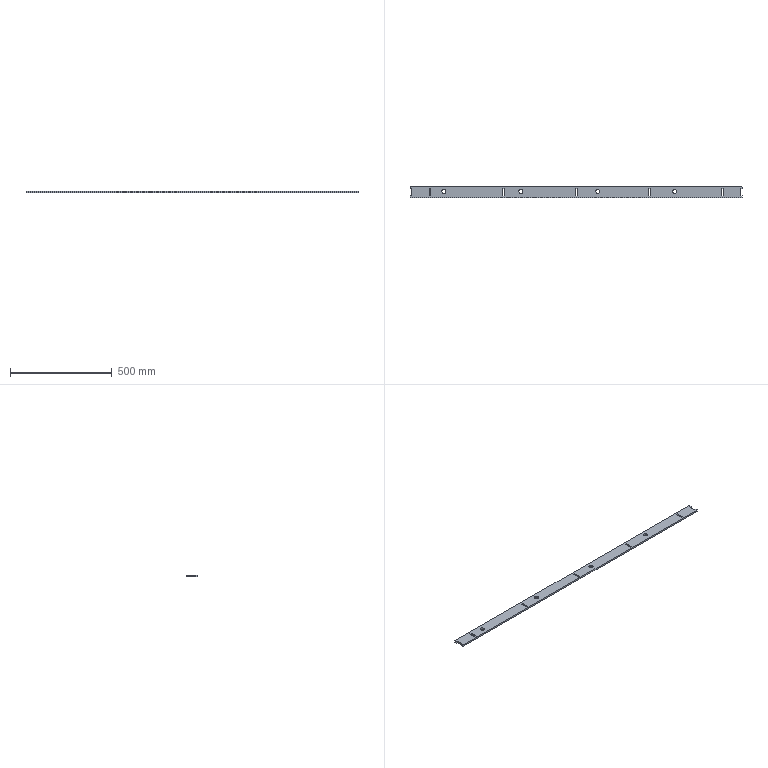Part | SolidWorks | features FlatPattern 1, SMBaseFlange 1, SheetMetal 1 | 1 solid | 42 faces | box 1635 x 55 x 8 mm | volume 693667 mm3 | plane 34 | cylinder 8 | commonest cylinder face diameters 20 x8
STEP:
#1=CARTESIAN_POINT('',(1294.,-523.,8.));
#2=VERTEX_POINT('',#1);
#3=CARTESIAN_POINT('',(1314.,-523.,8.));
#4=VERTEX_POINT('',#3);
#5=CARTESIAN_POINT('',(1304.,-523.,8.));
#6=DIRECTION('',(0.,0.,1.));
#7=DIRECTION('',(1.,0.,0.));
#8=AXIS2_PLACEMENT_3D('',#5,#6,#7);
#9=CIRCLE('',#8,10.);
#10=EDGE_CURVE('',#2,#4,#9,.T.);
#11=ORIENTED_EDGE('',*,*,#10,.T.);
#12=CARTESIAN_POINT('',(1314.,-523.,0.));
#13=VERTEX_POINT('',#12);
#14=CARTESIAN_POINT('',(1314.,-523.,8.));
#15=DIRECTION('',(0.,0.,-1.));
#16=VECTOR('',#15,1000.);
#17=LINE('',#14,#16);
#18=EDGE_CURVE('',#4,#13,#17,.T.);
#19=ORIENTED_EDGE('',*,*,#18,.T.);
#20=CARTESIAN_POINT('',(1294.,-523.,0.));
#21=VERTEX_POINT('',#20);
#22=CARTESIAN_POINT('',(1304.,-523.,0.));
#23=DIRECTION('',(0.,0.,1.));
#24=DIRECTION('',(1.,0.,0.));
#25=AXIS2_PLACEMENT_3D('',#22,#23,#24);
#26=CIRCLE('',#25,10.);
#27=EDGE_CURVE('',#21,#13,#26,.T.);
#28=ORIENTED_EDGE('',*,*,#27,.F.);
#29=CARTESIAN_POINT('',(1294.,-523.,8.));
#30=DIRECTION('',(0.,0.,-1.));
#31=VECTOR('',#30,1000.);
#32=LINE('',#29,#31);
#33=EDGE_CURVE('',#2,#21,#32,.T.);
#34=ORIENTED_EDGE('',*,*,#33,.F.);
#35=EDGE_LOOP('',(#11,#19,#28,#34));
#36=FACE_OUTER_BOUND('',#35,.T.);
#37=CARTESIAN_POINT('',(1304.,-523.,8.));
#38=DIRECTION('',(0.,0.,-1.));
#39=DIRECTION('',(-1.,0.,0.));
#40=AXIS2_PLACEMENT_3D('',#37,#38,#39);
#41=CYLINDRICAL_SURFACE('',#40,10.);
#42=ADVANCED_FACE('',(#36),#41,.F.);
#43=CARTESIAN_POINT('',(915.,-523.,8.));
#44=VERTEX_POINT('',#43);
#45=CARTESIAN_POINT('',(935.,-523.,8.));
#46=VERTEX_POINT('',#45);
#47=CARTESIAN_POINT('',(925.,-523.,8.));
#48=DIRECTION('',(0.,0.,1.));
#49=DIRECTION('',(1.,0.,0.));
#50=AXIS2_PLACEMENT_3D('',#47,#48,#49);
#51=CIRCLE('',#50,10.);
#52=EDGE_CURVE('',#44,#46,#51,.T.);
#53=ORIENTED_EDGE('',*,*,#52,.T.);
#54=CARTESIAN_POINT('',(935.,-523.,0.));
#55=VERTEX_POINT('',#54);
#56=CARTESIAN_POINT('',(935.,-523.,8.));
#57=DIRECTION('',(0.,0.,-1.));
#58=VECTOR('',#57,1000.);
#59=LINE('',#56,#58);
#60=EDGE_CURVE('',#46,#55,#59,.T.);
#61=ORIENTED_EDGE('',*,*,#60,.T.);
#62=CARTESIAN_POINT('',(915.,-523.,0.));
#63=VERTEX_POINT('',#62);
#64=CARTESIAN_POINT('',(925.,-523.,0.));
#65=DIRECTION('',(0.,0.,1.));
#66=DIRECTION('',(1.,0.,0.));
#67=AXIS2_PLACEMENT_3D('',#64,#65,#66);
#68=CIRCLE('',#67,10.);
#69=EDGE_CURVE('',#63,#55,#68,.T.);
#70=ORIENTED_EDGE('',*,*,#69,.F.);
#71=CARTESIAN_POINT('',(915.,-523.,8.));
#72=DIRECTION('',(0.,0.,-1.));
#73=VECTOR('',#72,1000.);
#74=LINE('',#71,#73);
#75=EDGE_CURVE('',#44,#63,#74,.T.);
#76=ORIENTED_EDGE('',*,*,#75,.F.);
#77=EDGE_LOOP('',(#53,#61,#70,#76));
#78=FACE_OUTER_BOUND('',#77,.T.);
#79=CARTESIAN_POINT('',(925.,-523.,8.));
#80=DIRECTION('',(0.,0.,-1.));
#81=DIRECTION('',(-1.,0.,0.));
#82=AXIS2_PLACEMENT_3D('',#79,#80,#81);
#83=CYLINDRICAL_SURFACE('',#82,10.);
#84=ADVANCED_FACE('',(#78),#83,.F.);
#85=CARTESIAN_POINT('',(536.,-523.,8.));
#86=VERTEX_POINT('',#85);
#87=CARTESIAN_POINT('',(556.,-523.,8.));
#88=VERTEX_POINT('',#87);
#89=CARTESIAN_POINT('',(546.,-523.,8.));
#90=DIRECTION('',(0.,0.,1.));
#91=DIRECTION('',(1.,0.,0.));
#92=AXIS2_PLACEMENT_3D('',#89,#90,#91);
#93=CIRCLE('',#92,10.);
#94=EDGE_CURVE('',#86,#88,#93,.T.);
#95=ORIENTED_EDGE('',*,*,#94,.T.);
#96=CARTESIAN_POINT('',(556.,-523.,0.));
#97=VERTEX_POINT('',#96);
#98=CARTESIAN_POINT('',(556.,-523.,8.));
#99=DIRECTION('',(0.,0.,-1.));
#100=VECTOR('',#99,1000.);
#101=LINE('',#98,#100);
#102=EDGE_CURVE('',#88,#97,#101,.T.);
#103=ORIENTED_EDGE('',*,*,#102,.T.);
#104=CARTESIAN_POINT('',(536.,-523.,0.));
#105=VERTEX_POINT('',#104);
#106=CARTESIAN_POINT('',(546.,-523.,0.));
#107=DIRECTION('',(0.,0.,1.));
#108=DIRECTION('',(1.,0.,0.));
#109=AXIS2_PLACEMENT_3D('',#106,#107,#108);
#110=CIRCLE('',#109,10.);
#111=EDGE_CURVE('',#105,#97,#110,.T.);
#112=ORIENTED_EDGE('',*,*,#111,.F.);
#113=CARTESIAN_POINT('',(536.,-523.,8.));
#114=DIRECTION('',(0.,0.,-1.));
#115=VECTOR('',#114,1000.);
#116=LINE('',#113,#115);
#117=EDGE_CURVE('',#86,#105,#116,.T.);
#118=ORIENTED_EDGE('',*,*,#117,.F.);
#119=EDGE_LOOP('',(#95,#103,#112,#118));
#120=FACE_OUTER_BOUND('',#119,.T.);
#121=CARTESIAN_POINT('',(546.,-523.,8.));
#122=DIRECTION('',(0.,0.,-1.));
#123=DIRECTION('',(-1.,0.,0.));
#124=AXIS2_PLACEMENT_3D('',#121,#122,#123);
#125=CYLINDRICAL_SURFACE('',#124,10.);
#126=ADVANCED_FACE('',(#120),#125,.F.);
#127=CARTESIAN_POINT('',(157.,-523.,8.));
#128=VERTEX_POINT('',#127);
#129=CARTESIAN_POINT('',(177.,-523.,8.));
#130=VERTEX_POINT('',#129);
#131=CARTESIAN_POINT('',(167.,-523.,8.));
#132=DIRECTION('',(0.,0.,1.));
#133=DIRECTION('',(1.,0.,0.));
#134=AXIS2_PLACEMENT_3D('',#131,#132,#133);
#135=CIRCLE('',#134,10.);
#136=EDGE_CURVE('',#128,#130,#135,.T.);
#137=ORIENTED_EDGE('',*,*,#136,.T.);
#138=CARTESIAN_POINT('',(177.,-523.,0.));
#139=VERTEX_POINT('',#138);
#140=CARTESIAN_POINT('',(177.,-523.,8.));
#141=DIRECTION('',(0.,0.,-1.));
#142=VECTOR('',#141,1000.);
#143=LINE('',#140,#142);
#144=EDGE_CURVE('',#130,#139,#143,.T.);
#145=ORIENTED_EDGE('',*,*,#144,.T.);
#146=CARTESIAN_POINT('',(157.,-523.,0.));
#147=VERTEX_POINT('',#146);
#148=CARTESIAN_POINT('',(167.,-523.,0.));
#149=DIRECTION('',(0.,0.,1.));
#150=DIRECTION('',(1.,0.,0.));
#151=AXIS2_PLACEMENT_3D('',#148,#149,#150);
#152=CIRCLE('',#151,10.);
#153=EDGE_CURVE('',#147,#139,#152,.T.);
#154=ORIENTED_EDGE('',*,*,#153,.F.);
#155=CARTESIAN_POINT('',(157.,-523.,8.));
#156=DIRECTION('',(0.,0.,-1.));
#157=VECTOR('',#156,1000.);
#158=LINE('',#155,#157);
#159=EDGE_CURVE('',#128,#147,#158,.T.);
#160=ORIENTED_EDGE('',*,*,#159,.F.);
#161=EDGE_LOOP('',(#137,#145,#154,#160));
#162=FACE_OUTER_BOUND('',#161,.T.);
#163=CARTESIAN_POINT('',(167.,-523.,8.));
#164=DIRECTION('',(0.,0.,-1.));
#165=DIRECTION('',(-1.,0.,0.));
#166=AXIS2_PLACEMENT_3D('',#163,#164,#165);
#167=CYLINDRICAL_SURFACE('',#166,10.);
#168=ADVANCED_FACE('',(#162),#167,.F.);
#169=CARTESIAN_POINT('',(1183.,-544.809,8.));
#170=VERTEX_POINT('',#169);
#171=CARTESIAN_POINT('',(1183.,-509.809,8.));
#172=VERTEX_POINT('',#171);
#173=CARTESIAN_POINT('',(1183.,-509.809,8.));
#174=DIRECTION('',(0.,1.,0.));
#175=VECTOR('',#174,1000.);
#176=LINE('',#173,#175);
#177=EDGE_CURVE('',#170,#172,#176,.T.);
#178=ORIENTED_EDGE('',*,*,#177,.F.);
#179=CARTESIAN_POINT('',(1175.,-544.809,8.));
#180=VERTEX_POINT('',#179);
#181=CARTESIAN_POINT('',(1183.,-544.809,8.));
#182=DIRECTION('',(1.,0.,0.));
#183=VECTOR('',#182,1000.);
#184=LINE('',#181,#183);
#185=EDGE_CURVE('',#180,#170,#184,.T.);
#186=ORIENTED_EDGE('',*,*,#185,.F.);
#187=CARTESIAN_POINT('',(1175.,-509.809,8.));
#188=VERTEX_POINT('',#187);
#189=CARTESIAN_POINT('',(1175.,-509.809,8.));
#190=DIRECTION('',(0.,-1.,0.));
#191=VECTOR('',#190,1000.);
#192=LINE('',#189,#191);
#193=EDGE_CURVE('',#188,#180,#192,.T.);
#194=ORIENTED_EDGE('',*,*,#193,.F.);
#195=CARTESIAN_POINT('',(1183.,-509.809,8.));
#196=DIRECTION('',(-1.,0.,0.));
#197=VECTOR('',#196,1000.);
#198=LINE('',#195,#197);
#199=EDGE_CURVE('',#172,#188,#198,.T.);
#200=ORIENTED_EDGE('',*,*,#199,.F.);
#201=EDGE_LOOP('',(#178,#186,#194,#200));
#202=FACE_BOUND('',#201,.T.);
#203=CARTESIAN_POINT('',(455.,-509.809,8.));
#204=VERTEX_POINT('',#203);
#205=CARTESIAN_POINT('',(455.,-544.809,8.));
#206=VERTEX_POINT('',#205);
#207=CARTESIAN_POINT('',(455.,-509.809,8.));
#208=DIRECTION('',(0.,-1.,0.));
#209=VECTOR('',#208,1000.);
#210=LINE('',#207,#209);
#211=EDGE_CURVE('',#204,#206,#210,.T.);
#212=ORIENTED_EDGE('',*,*,#211,.F.);
#213=CARTESIAN_POINT('',(463.,-509.809,8.));
#214=VERTEX_POINT('',#213);
#215=CARTESIAN_POINT('',(455.,-509.809,8.));
#216=DIRECTION('',(-1.,0.,0.));
#217=VECTOR('',#216,1000.);
#218=LINE('',#215,#217);
#219=EDGE_CURVE('',#214,#204,#218,.T.);
#220=ORIENTED_EDGE('',*,*,#219,.F.);
#221=CARTESIAN_POINT('',(463.,-544.809,8.));
#222=VERTEX_POINT('',#221);
#223=CARTESIAN_POINT('',(463.,-509.809,8.));
#224=DIRECTION('',(0.,1.,0.));
#225=VECTOR('',#224,1000.);
#226=LINE('',#223,#225);
#227=EDGE_CURVE('',#222,#214,#226,.T.);
#228=ORIENTED_EDGE('',*,*,#227,.F.);
#229=CARTESIAN_POINT('',(455.,-544.809,8.));
#230=DIRECTION('',(1.,0.,0.));
#231=VECTOR('',#230,1000.);
#232=LINE('',#229,#231);
#233=EDGE_CURVE('',#206,#222,#232,.T.);
#234=ORIENTED_EDGE('',*,*,#233,.F.);
#235=EDGE_LOOP('',(#212,#220,#228,#234));
#236=FACE_BOUND('',#235,.T.);
#237=ORIENTED_EDGE('',*,*,#10,.F.);
#238=CARTESIAN_POINT('',(1304.,-523.,8.));
#239=DIRECTION('',(0.,0.,1.));
#240=DIRECTION('',(1.,0.,0.));
#241=AXIS2_PLACEMENT_3D('',#238,#239,#240);
#242=CIRCLE('',#241,10.);
#243=EDGE_CURVE('',#4,#2,#242,.T.);
#244=ORIENTED_EDGE('',*,*,#243,.F.);
#245=EDGE_LOOP('',(#237,#244));
#246=FACE_BOUND('',#245,.T.);
#247=ORIENTED_EDGE('',*,*,#52,.F.);
#248=CARTESIAN_POINT('',(925.,-523.,8.));
#249=DIRECTION('',(0.,0.,1.));
#250=DIRECTION('',(1.,0.,0.));
#251=AXIS2_PLACEMENT_3D('',#248,#249,#250);
#252=CIRCLE('',#251,10.);
#253=EDGE_CURVE('',#46,#44,#252,.T.);
#254=ORIENTED_EDGE('',*,*,#253,.F.);
#255=EDGE_LOOP('',(#247,#254));
#256=FACE_BOUND('',#255,.T.);
#257=ORIENTED_EDGE('',*,*,#94,.F.);
#258=CARTESIAN_POINT('',(546.,-523.,8.));
#259=DIRECTION('',(0.,0.,1.));
#260=DIRECTION('',(1.,0.,0.));
#261=AXIS2_PLACEMENT_3D('',#258,#259,#260);
#262=CIRCLE('',#261,10.);
#263=EDGE_CURVE('',#88,#86,#262,.T.);
#264=ORIENTED_EDGE('',*,*,#263,.F.);
#265=EDGE_LOOP('',(#257,#264));
#266=FACE_BOUND('',#265,.T.);
#267=ORIENTED_EDGE('',*,*,#136,.F.);
#268=CARTESIAN_POINT('',(167.,-523.,8.));
#269=DIRECTION('',(0.,0.,1.));
#270=DIRECTION('',(1.,0.,0.));
#271=AXIS2_PLACEMENT_3D('',#268,#269,#270);
#272=CIRCLE('',#271,10.);
#273=EDGE_CURVE('',#130,#128,#272,.T.);
#274=ORIENTED_EDGE('',*,*,#273,.F.);
#275=EDGE_LOOP('',(#267,#274));
#276=FACE_BOUND('',#275,.T.);
#277=CARTESIAN_POINT('',(0.,-498.431,8.));
#278=VERTEX_POINT('',#277);
#279=CARTESIAN_POINT('',(0.,-509.809,8.));
#280=VERTEX_POINT('',#279);
#281=CARTESIAN_POINT('',(0.,-498.431,8.));
#282=DIRECTION('',(0.,-1.,0.));
#283=VECTOR('',#282,1000.);
#284=LINE('',#281,#283);
#285=EDGE_CURVE('',#278,#280,#284,.T.);
#286=ORIENTED_EDGE('',*,*,#285,.T.);
#287=CARTESIAN_POINT('',(8.,-509.809,8.));
#288=VERTEX_POINT('',#287);
#289=CARTESIAN_POINT('',(8.,-509.809,8.));
#290=DIRECTION('',(1.,0.,0.));
#291=VECTOR('',#290,1000.);
#292=LINE('',#289,#291);
#293=EDGE_CURVE('',#280,#288,#292,.T.);
#294=ORIENTED_EDGE('',*,*,#293,.T.);
#295=CARTESIAN_POINT('',(8.,-544.809,8.));
#296=VERTEX_POINT('',#295);
#297=CARTESIAN_POINT('',(8.,-509.809,8.));
#298=DIRECTION('',(0.,-1.,0.));
#299=VECTOR('',#298,1000.);
#300=LINE('',#297,#299);
#301=EDGE_CURVE('',#288,#296,#300,.T.);
#302=ORIENTED_EDGE('',*,*,#301,.T.);
#303=CARTESIAN_POINT('',(0.,-544.809,8.));
#304=VERTEX_POINT('',#303);
#305=CARTESIAN_POINT('',(8.,-544.809,8.));
#306=DIRECTION('',(-1.,0.,0.));
#307=VECTOR('',#306,1000.);
#308=LINE('',#305,#307);
#309=EDGE_CURVE('',#296,#304,#308,.T.);
#310=ORIENTED_EDGE('',*,*,#309,.T.);
#311=CARTESIAN_POINT('',(0.,-553.431,8.));
#312=VERTEX_POINT('',#311);
#313=CARTESIAN_POINT('',(0.,-544.809,8.));
#314=DIRECTION('',(0.,-1.,0.));
#315=VECTOR('',#314,1000.);
#316=LINE('',#313,#315);
#317=EDGE_CURVE('',#304,#312,#316,.T.);
#318=ORIENTED_EDGE('',*,*,#317,.T.);
#319=CARTESIAN_POINT('',(1635.,-553.431,8.));
#320=VERTEX_POINT('',#319);
#321=CARTESIAN_POINT('',(0.,-553.431,8.));
#322=DIRECTION('',(1.,0.,0.));
#323=VECTOR('',#322,1000.);
#324=LINE('',#321,#323);
#325=EDGE_CURVE('',#312,#320,#324,.T.);
#326=ORIENTED_EDGE('',*,*,#325,.T.);
#327=CARTESIAN_POINT('',(1635.,-544.809,8.));
#328=VERTEX_POINT('',#327);
#329=CARTESIAN_POINT('',(1635.,-544.809,8.));
#330=DIRECTION('',(0.,1.,0.));
#331=VECTOR('',#330,1000.);
#332=LINE('',#329,#331);
#333=EDGE_CURVE('',#320,#328,#332,.T.);
#334=ORIENTED_EDGE('',*,*,#333,.T.);
#335=CARTESIAN_POINT('',(1627.,-544.809,8.));
#336=VERTEX_POINT('',#335);
#337=CARTESIAN_POINT('',(1635.,-544.809,8.));
#338=DIRECTION('',(-1.,0.,0.));
#339=VECTOR('',#338,1000.);
#340=LINE('',#337,#339);
#341=EDGE_CURVE('',#328,#336,#340,.T.);
#342=ORIENTED_EDGE('',*,*,#341,.T.);
#343=CARTESIAN_POINT('',(1627.,-509.809,8.));
#344=VERTEX_POINT('',#343);
#345=CARTESIAN_POINT('',(1627.,-509.809,8.));
#346=DIRECTION('',(0.,1.,0.));
#347=VECTOR('',#346,1000.);
#348=LINE('',#345,#347);
#349=EDGE_CURVE('',#336,#344,#348,.T.);
#350=ORIENTED_EDGE('',*,*,#349,.T.);
#351=CARTESIAN_POINT('',(1635.,-509.809,8.));
#352=VERTEX_POINT('',#351);
#353=CARTESIAN_POINT('',(1635.,-509.809,8.));
#354=DIRECTION('',(1.,0.,0.));
#355=VECTOR('',#354,1000.);
#356=LINE('',#353,#355);
#357=EDGE_CURVE('',#344,#352,#356,.T.);
#358=ORIENTED_EDGE('',*,*,#357,.T.);
#359=CARTESIAN_POINT('',(1635.,-498.431,8.));
#360=VERTEX_POINT('',#359);
#361=CARTESIAN_POINT('',(1635.,-498.431,8.));
#362=DIRECTION('',(0.,1.,0.));
#363=VECTOR('',#362,1000.);
#364=LINE('',#361,#363);
#365=EDGE_CURVE('',#352,#360,#364,.T.);
#366=ORIENTED_EDGE('',*,*,#365,.T.);
#367=CARTESIAN_POINT('',(0.,-498.431,8.));
#368=DIRECTION('',(-1.,0.,0.));
#369=VECTOR('',#368,1000.);
#370=LINE('',#367,#369);
#371=EDGE_CURVE('',#360,#278,#370,.T.);
#372=ORIENTED_EDGE('',*,*,#371,.T.);
#373=EDGE_LOOP('',(#286,#294,#302,#310,#318,#326,#334,#342,#350,#358,#366,#372));
#374=FACE_OUTER_BOUND('',#373,.T.);
#375=CARTESIAN_POINT('',(95.,-509.809,8.));
#376=VERTEX_POINT('',#375);
#377=CARTESIAN_POINT('',(95.,-544.809,8.));
#378=VERTEX_POINT('',#377);
#379=CARTESIAN_POINT('',(95.,-544.809,8.));
#380=DIRECTION('',(0.,-1.,0.));
#381=VECTOR('',#380,1000.);
#382=LINE('',#379,#381);
#383=EDGE_CURVE('',#376,#378,#382,.T.);
#384=ORIENTED_EDGE('',*,*,#383,.F.);
#385=CARTESIAN_POINT('',(103.,-509.809,8.));
#386=VERTEX_POINT('',#385);
#387=CARTESIAN_POINT('',(95.,-509.809,8.));
#388=DIRECTION('',(-1.,0.,0.));
#389=VECTOR('',#388,1000.);
#390=LINE('',#387,#389);
#391=EDGE_CURVE('',#386,#376,#390,.T.);
#392=ORIENTED_EDGE('',*,*,#391,.F.);
#393=CARTESIAN_POINT('',(103.,-544.809,8.));
#394=VERTEX_POINT('',#393);
#395=CARTESIAN_POINT('',(103.,-544.809,8.));
#396=DIRECTION('',(0.,1.,0.));
#397=VECTOR('',#396,1000.);
#398=LINE('',#395,#397);
#399=EDGE_CURVE('',#394,#386,#398,.T.);
#400=ORIENTED_EDGE('',*,*,#399,.F.);
#401=CARTESIAN_POINT('',(95.,-544.809,8.));
#402=DIRECTION('',(1.,0.,0.));
#403=VECTOR('',#402,1000.);
#404=LINE('',#401,#403);
#405=EDGE_CURVE('',#378,#394,#404,.T.);
#406=ORIENTED_EDGE('',*,*,#405,.F.);
#407=EDGE_LOOP('',(#384,#392,#400,#406));
#408=FACE_BOUND('',#407,.T.);
#409=CARTESIAN_POINT('',(823.,-544.809,8.));
#410=VERTEX_POINT('',#409);
#411=CARTESIAN_POINT('',(823.,-509.809,8.));
#412=VERTEX_POINT('',#411);
#413=CARTESIAN_POINT('',(823.,-509.809,8.));
#414=DIRECTION('',(0.,1.,0.));
#415=VECTOR('',#414,1000.);
#416=LINE('',#413,#415);
#417=EDGE_CURVE('',#410,#412,#416,.T.);
#418=ORIENTED_EDGE('',*,*,#417,.F.);
#419=CARTESIAN_POINT('',(815.,-544.809,8.));
#420=VERTEX_POINT('',#419);
#421=CARTESIAN_POINT('',(823.,-544.809,8.));
#422=DIRECTION('',(1.,0.,0.));
#423=VECTOR('',#422,1000.);
#424=LINE('',#421,#423);
#425=EDGE_CURVE('',#420,#410,#424,.T.);
#426=ORIENTED_EDGE('',*,*,#425,.F.);
#427=CARTESIAN_POINT('',(815.,-509.809,8.));
#428=VERTEX_POINT('',#427);
#429=CARTESIAN_POINT('',(815.,-509.809,8.));
#430=DIRECTION('',(0.,-1.,0.));
#431=VECTOR('',#430,1000.);
#432=LINE('',#429,#431);
#433=EDGE_CURVE('',#428,#420,#432,.T.);
#434=ORIENTED_EDGE('',*,*,#433,.F.);
#435=CARTESIAN_POINT('',(823.,-509.809,8.));
#436=DIRECTION('',(-1.,0.,0.));
#437=VECTOR('',#436,1000.);
#438=LINE('',#435,#437);
#439=EDGE_CURVE('',#412,#428,#438,.T.);
#440=ORIENTED_EDGE('',*,*,#439,.F.);
#441=EDGE_LOOP('',(#418,#426,#434,#440));
#442=FACE_BOUND('',#441,.T.);
#443=CARTESIAN_POINT('',(1543.,-544.809,8.));
#444=VERTEX_POINT('',#443);
#445=CARTESIAN_POINT('',(1543.,-509.809,8.));
#446=VERTEX_POINT('',#445);
#447=CARTESIAN_POINT('',(1543.,-509.809,8.));
#448=DIRECTION('',(0.,1.,0.));
#449=VECTOR('',#448,1000.);
#450=LINE('',#447,#449);
#451=EDGE_CURVE('',#444,#446,#450,.T.);
#452=ORIENTED_EDGE('',*,*,#451,.F.);
#453=CARTESIAN_POINT('',(1535.,-544.809,8.));
#454=VERTEX_POINT('',#453);
#455=CARTESIAN_POINT('',(1543.,-544.809,8.));
#456=DIRECTION('',(1.,0.,0.));
#457=VECTOR('',#456,1000.);
#458=LINE('',#455,#457);
#459=EDGE_CURVE('',#454,#444,#458,.T.);
#460=ORIENTED_EDGE('',*,*,#459,.F.);
#461=CARTESIAN_POINT('',(1535.,-509.809,8.));
#462=VERTEX_POINT('',#461);
#463=CARTESIAN_POINT('',(1535.,-509.809,8.));
#464=DIRECTION('',(0.,-1.,0.));
#465=VECTOR('',#464,1000.);
#466=LINE('',#463,#465);
#467=EDGE_CURVE('',#462,#454,#466,.T.);
#468=ORIENTED_EDGE('',*,*,#467,.F.);
#469=CARTESIAN_POINT('',(1543.,-509.809,8.));
#470=DIRECTION('',(-1.,0.,0.));
#471=VECTOR('',#470,1000.);
#472=LINE('',#469,#471);
#473=EDGE_CURVE('',#446,#462,#472,.T.);
#474=ORIENTED_EDGE('',*,*,#473,.F.);
#475=EDGE_LOOP('',(#452,#460,#468,#474));
#476=FACE_BOUND('',#475,.T.);
#477=CARTESIAN_POINT('',(0.,0.,8.));
#478=DIRECTION('',(0.,0.,-1.));
#479=DIRECTION('',(-1.,0.,0.));
#480=AXIS2_PLACEMENT_3D('',#477,#478,#479);
#481=PLANE('',#480);
#482=ADVANCED_FACE('',(#202,#236,#246,#256,#266,#276,#374,#408,#442,#476),#481,.F.);
#483=ORIENTED_EDGE('',*,*,#69,.T.);
#484=CARTESIAN_POINT('',(925.,-523.,0.));
#485=DIRECTION('',(0.,0.,1.));
#486=DIRECTION('',(1.,0.,0.));
#487=AXIS2_PLACEMENT_3D('',#484,#485,#486);
#488=CIRCLE('',#487,10.);
#489=EDGE_CURVE('',#55,#63,#488,.T.);
#490=ORIENTED_EDGE('',*,*,#489,.T.);
#491=EDGE_LOOP('',(#483,#490));
#492=FACE_BOUND('',#491,.T.);
#493=ORIENTED_EDGE('',*,*,#153,.T.);
#494=CARTESIAN_POINT('',(167.,-523.,0.));
#495=DIRECTION('',(0.,0.,1.));
#496=DIRECTION('',(1.,0.,0.));
#497=AXIS2_PLACEMENT_3D('',#494,#495,#496);
#498=CIRCLE('',#497,10.);
#499=EDGE_CURVE('',#139,#147,#498,.T.);
#500=ORIENTED_EDGE('',*,*,#499,.T.);
#501=EDGE_LOOP('',(#493,#500));
#502=FACE_BOUND('',#501,.T.);
#503=CARTESIAN_POINT('',(0.,-498.431,0.));
#504=VERTEX_POINT('',#503);
#505=CARTESIAN_POINT('',(0.,-509.809,0.));
#506=VERTEX_POINT('',#505);
#507=CARTESIAN_POINT('',(0.,-498.431,0.));
#508=DIRECTION('',(0.,-1.,0.));
#509=VECTOR('',#508,1000.);
#510=LINE('',#507,#509);
#511=EDGE_CURVE('',#504,#506,#510,.T.);
#512=ORIENTED_EDGE('',*,*,#511,.F.);
#513=CARTESIAN_POINT('',(1635.,-498.431,0.));
#514=VERTEX_POINT('',#513);
#515=CARTESIAN_POINT('',(0.,-498.431,0.));
#516=DIRECTION('',(-1.,0.,0.));
#517=VECTOR('',#516,1000.);
#518=LINE('',#515,#517);
#519=EDGE_CURVE('',#514,#504,#518,.T.);
#520=ORIENTED_EDGE('',*,*,#519,.F.);
#521=CARTESIAN_POINT('',(1635.,-509.809,0.));
#522=VERTEX_POINT('',#521);
#523=CARTESIAN_POINT('',(1635.,-498.431,0.));
#524=DIRECTION('',(0.,1.,0.));
#525=VECTOR('',#524,1000.);
#526=LINE('',#523,#525);
#527=EDGE_CURVE('',#522,#514,#526,.T.);
#528=ORIENTED_EDGE('',*,*,#527,.F.);
#529=CARTESIAN_POINT('',(1627.,-509.809,0.));
#530=VERTEX_POINT('',#529);
#531=CARTESIAN_POINT('',(1635.,-509.809,0.));
#532=DIRECTION('',(1.,0.,0.));
#533=VECTOR('',#532,1000.);
#534=LINE('',#531,#533);
#535=EDGE_CURVE('',#530,#522,#534,.T.);
#536=ORIENTED_EDGE('',*,*,#535,.F.);
#537=CARTESIAN_POINT('',(1627.,-544.809,0.));
#538=VERTEX_POINT('',#537);
#539=CARTESIAN_POINT('',(1627.,-509.809,0.));
#540=DIRECTION('',(0.,1.,0.));
#541=VECTOR('',#540,1000.);
#542=LINE('',#539,#541);
#543=EDGE_CURVE('',#538,#530,#542,.T.);
#544=ORIENTED_EDGE('',*,*,#543,.F.);
#545=CARTESIAN_POINT('',(1635.,-544.809,0.));
#546=VERTEX_POINT('',#545);
#547=CARTESIAN_POINT('',(1635.,-544.809,0.));
#548=DIRECTION('',(-1.,0.,0.));
#549=VECTOR('',#548,1000.);
#550=LINE('',#547,#549);
#551=EDGE_CURVE('',#546,#538,#550,.T.);
#552=ORIENTED_EDGE('',*,*,#551,.F.);
#553=CARTESIAN_POINT('',(1635.,-553.431,0.));
#554=VERTEX_POINT('',#553);
#555=CARTESIAN_POINT('',(1635.,-544.809,0.));
#556=DIRECTION('',(0.,1.,0.));
#557=VECTOR('',#556,1000.);
#558=LINE('',#555,#557);
#559=EDGE_CURVE('',#554,#546,#558,.T.);
#560=ORIENTED_EDGE('',*,*,#559,.F.);
#561=CARTESIAN_POINT('',(0.,-553.431,0.));
#562=VERTEX_POINT('',#561);
#563=CARTESIAN_POINT('',(0.,-553.431,0.));
#564=DIRECTION('',(1.,0.,0.));
#565=VECTOR('',#564,1000.);
#566=LINE('',#563,#565);
#567=EDGE_CURVE('',#562,#554,#566,.T.);
#568=ORIENTED_EDGE('',*,*,#567,.F.);
#569=CARTESIAN_POINT('',(0.,-544.809,0.));
#570=VERTEX_POINT('',#569);
#571=CARTESIAN_POINT('',(0.,-544.809,0.));
#572=DIRECTION('',(0.,-1.,0.));
#573=VECTOR('',#572,1000.);
#574=LINE('',#571,#573);
#575=EDGE_CURVE('',#570,#562,#574,.T.);
#576=ORIENTED_EDGE('',*,*,#575,.F.);
#577=CARTESIAN_POINT('',(8.,-544.809,0.));
#578=VERTEX_POINT('',#577);
#579=CARTESIAN_POINT('',(8.,-544.809,0.));
#580=DIRECTION('',(-1.,0.,0.));
#581=VECTOR('',#580,1000.);
#582=LINE('',#579,#581);
#583=EDGE_CURVE('',#578,#570,#582,.T.);
#584=ORIENTED_EDGE('',*,*,#583,.F.);
#585=CARTESIAN_POINT('',(8.,-509.809,0.));
#586=VERTEX_POINT('',#585);
#587=CARTESIAN_POINT('',(8.,-509.809,0.));
#588=DIRECTION('',(0.,-1.,0.));
#589=VECTOR('',#588,1000.);
#590=LINE('',#587,#589);
#591=EDGE_CURVE('',#586,#578,#590,.T.);
#592=ORIENTED_EDGE('',*,*,#591,.F.);
#593=CARTESIAN_POINT('',(8.,-509.809,0.));
#594=DIRECTION('',(1.,0.,0.));
#595=VECTOR('',#594,1000.);
#596=LINE('',#593,#595);
#597=EDGE_CURVE('',#506,#586,#596,.T.);
#598=ORIENTED_EDGE('',*,*,#597,.F.);
#599=EDGE_LOOP('',(#512,#520,#528,#536,#544,#552,#560,#568,#576,#584,#592,#598));
#600=FACE_OUTER_BOUND('',#599,.T.);
#601=ORIENTED_EDGE('',*,*,#111,.T.);
#602=CARTESIAN_POINT('',(546.,-523.,0.));
#603=DIRECTION('',(0.,0.,1.));
#604=DIRECTION('',(1.,0.,0.));
#605=AXIS2_PLACEMENT_3D('',#602,#603,#604);
#606=CIRCLE('',#605,10.);
#607=EDGE_CURVE('',#97,#105,#606,.T.);
#608=ORIENTED_EDGE('',*,*,#607,.T.);
#609=EDGE_LOOP('',(#601,#608));
#610=FACE_BOUND('',#609,.T.);
#611=ORIENTED_EDGE('',*,*,#27,.T.);
#612=CARTESIAN_POINT('',(1304.,-523.,0.));
#613=DIRECTION('',(0.,0.,1.));
#614=DIRECTION('',(1.,0.,0.));
#615=AXIS2_PLACEMENT_3D('',#612,#613,#614);
#616=CIRCLE('',#615,10.);
#617=EDGE_CURVE('',#13,#21,#616,.T.);
#618=ORIENTED_EDGE('',*,*,#617,.T.);
#619=EDGE_LOOP('',(#611,#618));
#620=FACE_BOUND('',#619,.T.);
#621=CARTESIAN_POINT('',(103.,-509.809,0.));
#622=VERTEX_POINT('',#621);
#623=CARTESIAN_POINT('',(95.,-509.809,0.));
#624=VERTEX_POINT('',#623);
#625=CARTESIAN_POINT('',(95.,-509.809,0.));
#626=DIRECTION('',(-1.,0.,0.));
#627=VECTOR('',#626,1000.);
#628=LINE('',#625,#627);
#629=EDGE_CURVE('',#622,#624,#628,.T.);
#630=ORIENTED_EDGE('',*,*,#629,.T.);
#631=CARTESIAN_POINT('',(95.,-544.809,0.));
#632=VERTEX_POINT('',#631);
#633=CARTESIAN_POINT('',(95.,-544.809,0.));
#634=DIRECTION('',(0.,-1.,0.));
#635=VECTOR('',#634,1000.);
#636=LINE('',#633,#635);
#637=EDGE_CURVE('',#624,#632,#636,.T.);
#638=ORIENTED_EDGE('',*,*,#637,.T.);
#639=CARTESIAN_POINT('',(103.,-544.809,0.));
#640=VERTEX_POINT('',#639);
#641=CARTESIAN_POINT('',(95.,-544.809,0.));
#642=DIRECTION('',(1.,0.,0.));
#643=VECTOR('',#642,1000.);
#644=LINE('',#641,#643);
#645=EDGE_CURVE('',#632,#640,#644,.T.);
#646=ORIENTED_EDGE('',*,*,#645,.T.);
#647=CARTESIAN_POINT('',(103.,-544.809,0.));
#648=DIRECTION('',(0.,1.,0.));
#649=VECTOR('',#648,1000.);
#650=LINE('',#647,#649);
#651=EDGE_CURVE('',#640,#622,#650,.T.);
#652=ORIENTED_EDGE('',*,*,#651,.T.);
#653=EDGE_LOOP('',(#630,#638,#646,#652));
#654=FACE_BOUND('',#653,.T.);
#655=CARTESIAN_POINT('',(463.,-509.809,0.));
#656=VERTEX_POINT('',#655);
#657=CARTESIAN_POINT('',(455.,-509.809,0.));
#658=VERTEX_POINT('',#657);
#659=CARTESIAN_POINT('',(455.,-509.809,0.));
#660=DIRECTION('',(-1.,0.,0.));
#661=VECTOR('',#660,1000.);
#662=LINE('',#659,#661);
#663=EDGE_CURVE('',#656,#658,#662,.T.);
#664=ORIENTED_EDGE('',*,*,#663,.T.);
#665=CARTESIAN_POINT('',(455.,-544.809,0.));
#666=VERTEX_POINT('',#665);
#667=CARTESIAN_POINT('',(455.,-509.809,0.));
#668=DIRECTION('',(0.,-1.,0.));
#669=VECTOR('',#668,1000.);
#670=LINE('',#667,#669);
#671=EDGE_CURVE('',#658,#666,#670,.T.);
#672=ORIENTED_EDGE('',*,*,#671,.T.);
#673=CARTESIAN_POINT('',(463.,-544.809,0.));
#674=VERTEX_POINT('',#673);
#675=CARTESIAN_POINT('',(455.,-544.809,0.));
#676=DIRECTION('',(1.,0.,0.));
#677=VECTOR('',#676,1000.);
#678=LINE('',#675,#677);
#679=EDGE_CURVE('',#666,#674,#678,.T.);
#680=ORIENTED_EDGE('',*,*,#679,.T.);
#681=CARTESIAN_POINT('',(463.,-509.809,0.));
#682=DIRECTION('',(0.,1.,0.));
#683=VECTOR('',#682,1000.);
#684=LINE('',#681,#683);
#685=EDGE_CURVE('',#674,#656,#684,.T.);
#686=ORIENTED_EDGE('',*,*,#685,.T.);
#687=EDGE_LOOP('',(#664,#672,#680,#686));
#688=FACE_BOUND('',#687,.T.);
#689=CARTESIAN_POINT('',(815.,-544.809,0.));
#690=VERTEX_POINT('',#689);
#691=CARTESIAN_POINT('',(823.,-544.809,0.));
#692=VERTEX_POINT('',#691);
#693=CARTESIAN_POINT('',(823.,-544.809,0.));
#694=DIRECTION('',(1.,0.,0.));
#695=VECTOR('',#694,1000.);
#696=LINE('',#693,#695);
#697=EDGE_CURVE('',#690,#692,#696,.T.);
#698=ORIENTED_EDGE('',*,*,#697,.T.);
#699=CARTESIAN_POINT('',(823.,-509.809,0.));
#700=VERTEX_POINT('',#699);
#701=CARTESIAN_POINT('',(823.,-509.809,0.));
#702=DIRECTION('',(0.,1.,0.));
#703=VECTOR('',#702,1000.);
#704=LINE('',#701,#703);
#705=EDGE_CURVE('',#692,#700,#704,.T.);
#706=ORIENTED_EDGE('',*,*,#705,.T.);
#707=CARTESIAN_POINT('',(815.,-509.809,0.));
#708=VERTEX_POINT('',#707);
#709=CARTESIAN_POINT('',(823.,-509.809,0.));
#710=DIRECTION('',(-1.,0.,0.));
#711=VECTOR('',#710,1000.);
#712=LINE('',#709,#711);
#713=EDGE_CURVE('',#700,#708,#712,.T.);
#714=ORIENTED_EDGE('',*,*,#713,.T.);
#715=CARTESIAN_POINT('',(815.,-509.809,0.));
#716=DIRECTION('',(0.,-1.,0.));
#717=VECTOR('',#716,1000.);
#718=LINE('',#715,#717);
#719=EDGE_CURVE('',#708,#690,#718,.T.);
#720=ORIENTED_EDGE('',*,*,#719,.T.);
#721=EDGE_LOOP('',(#698,#706,#714,#720));
#722=FACE_BOUND('',#721,.T.);
#723=CARTESIAN_POINT('',(1175.,-544.809,0.));
#724=VERTEX_POINT('',#723);
#725=CARTESIAN_POINT('',(1183.,-544.809,0.));
#726=VERTEX_POINT('',#725);
#727=CARTESIAN_POINT('',(1183.,-544.809,0.));
#728=DIRECTION('',(1.,0.,0.));
#729=VECTOR('',#728,1000.);
#730=LINE('',#727,#729);
#731=EDGE_CURVE('',#724,#726,#730,.T.);
#732=ORIENTED_EDGE('',*,*,#731,.T.);
#733=CARTESIAN_POINT('',(1183.,-509.809,0.));
#734=VERTEX_POINT('',#733);
#735=CARTESIAN_POINT('',(1183.,-509.809,0.));
#736=DIRECTION('',(0.,1.,0.));
#737=VECTOR('',#736,1000.);
#738=LINE('',#735,#737);
#739=EDGE_CURVE('',#726,#734,#738,.T.);
#740=ORIENTED_EDGE('',*,*,#739,.T.);
#741=CARTESIAN_POINT('',(1175.,-509.809,0.));
#742=VERTEX_POINT('',#741);
#743=CARTESIAN_POINT('',(1183.,-509.809,0.));
#744=DIRECTION('',(-1.,0.,0.));
#745=VECTOR('',#744,1000.);
#746=LINE('',#743,#745);
#747=EDGE_CURVE('',#734,#742,#746,.T.);
#748=ORIENTED_EDGE('',*,*,#747,.T.);
#749=CARTESIAN_POINT('',(1175.,-509.809,0.));
#750=DIRECTION('',(0.,-1.,0.));
#751=VECTOR('',#750,1000.);
#752=LINE('',#749,#751);
#753=EDGE_CURVE('',#742,#724,#752,.T.);
#754=ORIENTED_EDGE('',*,*,#753,.T.);
#755=EDGE_LOOP('',(#732,#740,#748,#754));
#756=FACE_BOUND('',#755,.T.);
#757=CARTESIAN_POINT('',(1535.,-544.809,0.));
#758=VERTEX_POINT('',#757);
#759=CARTESIAN_POINT('',(1543.,-544.809,0.));
#760=VERTEX_POINT('',#759);
#761=CARTESIAN_POINT('',(1543.,-544.809,0.));
#762=DIRECTION('',(1.,0.,0.));
#763=VECTOR('',#762,1000.);
#764=LINE('',#761,#763);
#765=EDGE_CURVE('',#758,#760,#764,.T.);
#766=ORIENTED_EDGE('',*,*,#765,.T.);
#767=CARTESIAN_POINT('',(1543.,-509.809,0.));
#768=VERTEX_POINT('',#767);
#769=CARTESIAN_POINT('',(1543.,-509.809,0.));
#770=DIRECTION('',(0.,1.,0.));
#771=VECTOR('',#770,1000.);
#772=LINE('',#769,#771);
#773=EDGE_CURVE('',#760,#768,#772,.T.);
#774=ORIENTED_EDGE('',*,*,#773,.T.);
#775=CARTESIAN_POINT('',(1535.,-509.809,0.));
#776=VERTEX_POINT('',#775);
#777=CARTESIAN_POINT('',(1543.,-509.809,0.));
#778=DIRECTION('',(-1.,0.,0.));
#779=VECTOR('',#778,1000.);
#780=LINE('',#777,#779);
#781=EDGE_CURVE('',#768,#776,#780,.T.);
#782=ORIENTED_EDGE('',*,*,#781,.T.);
#783=CARTESIAN_POINT('',(1535.,-509.809,0.));
#784=DIRECTION('',(0.,-1.,0.));
#785=VECTOR('',#784,1000.);
#786=LINE('',#783,#785);
#787=EDGE_CURVE('',#776,#758,#786,.T.);
#788=ORIENTED_EDGE('',*,*,#787,.T.);
#789=EDGE_LOOP('',(#766,#774,#782,#788));
#790=FACE_BOUND('',#789,.T.);
#791=CARTESIAN_POINT('',(0.,0.,0.));
#792=DIRECTION('',(0.,0.,-1.));
#793=DIRECTION('',(-1.,0.,0.));
#794=AXIS2_PLACEMENT_3D('',#791,#792,#793);
#795=PLANE('',#794);
#796=ADVANCED_FACE('',(#492,#502,#600,#610,#620,#654,#688,#722,#756,#790),#795,.T.);
#797=ORIENTED_EDGE('',*,*,#511,.T.);
#798=CARTESIAN_POINT('',(0.,-509.809,8.));
#799=DIRECTION('',(0.,0.,-1.));
#800=VECTOR('',#799,1000.);
#801=LINE('',#798,#800);
#802=EDGE_CURVE('',#280,#506,#801,.T.);
#803=ORIENTED_EDGE('',*,*,#802,.F.);
#804=ORIENTED_EDGE('',*,*,#285,.F.);
#805=CARTESIAN_POINT('',(0.,-498.431,8.));
#806=DIRECTION('',(0.,0.,-1.));
#807=VECTOR('',#806,1000.);
#808=LINE('',#805,#807);
#809=EDGE_CURVE('',#278,#504,#808,.T.);
#810=ORIENTED_EDGE('',*,*,#809,.T.);
#811=EDGE_LOOP('',(#797,#803,#804,#810));
#812=FACE_OUTER_BOUND('',#811,.T.);
#813=CARTESIAN_POINT('',(0.,-498.431,8.));
#814=DIRECTION('',(1.,0.,0.));
#815=DIRECTION('',(0.,1.,0.));
#816=AXIS2_PLACEMENT_3D('',#813,#814,#815);
#817=PLANE('',#816);
#818=ADVANCED_FACE('',(#812),#817,.F.);
#819=ORIENTED_EDGE('',*,*,#597,.T.);
#820=CARTESIAN_POINT('',(8.,-509.809,8.));
#821=DIRECTION('',(0.,0.,-1.));
#822=VECTOR('',#821,1000.);
#823=LINE('',#820,#822);
#824=EDGE_CURVE('',#288,#586,#823,.T.);
#825=ORIENTED_EDGE('',*,*,#824,.F.);
#826=ORIENTED_EDGE('',*,*,#293,.F.);
#827=ORIENTED_EDGE('',*,*,#802,.T.);
#828=EDGE_LOOP('',(#819,#825,#826,#827));
#829=FACE_OUTER_BOUND('',#828,.T.);
#830=CARTESIAN_POINT('',(8.,-509.809,8.));
#831=DIRECTION('',(0.,1.,0.));
#832=DIRECTION('',(0.,0.,1.));
#833=AXIS2_PLACEMENT_3D('',#830,#831,#832);
#834=PLANE('',#833);
#835=ADVANCED_FACE('',(#829),#834,.F.);
#836=ORIENTED_EDGE('',*,*,#591,.T.);
#837=CARTESIAN_POINT('',(8.,-544.809,8.));
#838=DIRECTION('',(0.,0.,-1.));
#839=VECTOR('',#838,1000.);
#840=LINE('',#837,#839);
#841=EDGE_CURVE('',#296,#578,#840,.T.);
#842=ORIENTED_EDGE('',*,*,#841,.F.);
#843=ORIENTED_EDGE('',*,*,#301,.F.);
#844=ORIENTED_EDGE('',*,*,#824,.T.);
#845=EDGE_LOOP('',(#836,#842,#843,#844));
#846=FACE_OUTER_BOUND('',#845,.T.);
#847=CARTESIAN_POINT('',(8.,-509.809,8.));
#848=DIRECTION('',(1.,0.,0.));
#849=DIRECTION('',(0.,0.,-1.));
#850=AXIS2_PLACEMENT_3D('',#847,#848,#849);
#851=PLANE('',#850);
#852=ADVANCED_FACE('',(#846),#851,.F.);
#853=ORIENTED_EDGE('',*,*,#583,.T.);
#854=CARTESIAN_POINT('',(0.,-544.809,8.));
#855=DIRECTION('',(0.,0.,-1.));
#856=VECTOR('',#855,1000.);
#857=LINE('',#854,#856);
#858=EDGE_CURVE('',#304,#570,#857,.T.);
#859=ORIENTED_EDGE('',*,*,#858,.F.);
#860=ORIENTED_EDGE('',*,*,#309,.F.);
#861=ORIENTED_EDGE('',*,*,#841,.T.);
#862=EDGE_LOOP('',(#853,#859,#860,#861));
#863=FACE_OUTER_BOUND('',#862,.T.);
#864=CARTESIAN_POINT('',(8.,-544.809,8.));
#865=DIRECTION('',(0.,-1.,0.));
#866=DIRECTION('',(0.,0.,-1.));
#867=AXIS2_PLACEMENT_3D('',#864,#865,#866);
#868=PLANE('',#867);
#869=ADVANCED_FACE('',(#863),#868,.F.);
#870=ORIENTED_EDGE('',*,*,#575,.T.);
#871=CARTESIAN_POINT('',(0.,-553.431,8.));
#872=DIRECTION('',(0.,0.,-1.));
#873=VECTOR('',#872,1000.);
#874=LINE('',#871,#873);
#875=EDGE_CURVE('',#312,#562,#874,.T.);
#876=ORIENTED_EDGE('',*,*,#875,.F.);
#877=ORIENTED_EDGE('',*,*,#317,.F.);
#878=ORIENTED_EDGE('',*,*,#858,.T.);
#879=EDGE_LOOP('',(#870,#876,#877,#878));
#880=FACE_OUTER_BOUND('',#879,.T.);
#881=CARTESIAN_POINT('',(0.,-544.809,8.));
#882=DIRECTION('',(1.,0.,0.));
#883=DIRECTION('',(0.,1.,0.));
#884=AXIS2_PLACEMENT_3D('',#881,#882,#883);
#885=PLANE('',#884);
#886=ADVANCED_FACE('',(#880),#885,.F.);
#887=ORIENTED_EDGE('',*,*,#567,.T.);
#888=CARTESIAN_POINT('',(1635.,-553.431,8.));
#889=DIRECTION('',(0.,0.,-1.));
#890=VECTOR('',#889,1000.);
#891=LINE('',#888,#890);
#892=EDGE_CURVE('',#320,#554,#891,.T.);
#893=ORIENTED_EDGE('',*,*,#892,.F.);
#894=ORIENTED_EDGE('',*,*,#325,.F.);
#895=ORIENTED_EDGE('',*,*,#875,.T.);
#896=EDGE_LOOP('',(#887,#893,#894,#895));
#897=FACE_OUTER_BOUND('',#896,.T.);
#898=CARTESIAN_POINT('',(0.,-553.431,8.));
#899=DIRECTION('',(0.,1.,0.));
#900=DIRECTION('',(0.,0.,1.));
#901=AXIS2_PLACEMENT_3D('',#898,#899,#900);
#902=PLANE('',#901);
#903=ADVANCED_FACE('',(#897),#902,.F.);
#904=ORIENTED_EDGE('',*,*,#559,.T.);
#905=CARTESIAN_POINT('',(1635.,-544.809,8.));
#906=DIRECTION('',(0.,0.,-1.));
#907=VECTOR('',#906,1000.);
#908=LINE('',#905,#907);
#909=EDGE_CURVE('',#328,#546,#908,.T.);
#910=ORIENTED_EDGE('',*,*,#909,.F.);
#911=ORIENTED_EDGE('',*,*,#333,.F.);
#912=ORIENTED_EDGE('',*,*,#892,.T.);
#913=EDGE_LOOP('',(#904,#910,#911,#912));
#914=FACE_OUTER_BOUND('',#913,.T.);
#915=CARTESIAN_POINT('',(1635.,-544.809,8.));
#916=DIRECTION('',(-1.,0.,0.));
#917=DIRECTION('',(0.,0.,1.));
#918=AXIS2_PLACEMENT_3D('',#915,#916,#917);
#919=PLANE('',#918);
#920=ADVANCED_FACE('',(#914),#919,.F.);
#921=ORIENTED_EDGE('',*,*,#551,.T.);
#922=CARTESIAN_POINT('',(1627.,-544.809,8.));
#923=DIRECTION('',(0.,0.,-1.));
#924=VECTOR('',#923,1000.);
#925=LINE('',#922,#924);
#926=EDGE_CURVE('',#336,#538,#925,.T.);
#927=ORIENTED_EDGE('',*,*,#926,.F.);
#928=ORIENTED_EDGE('',*,*,#341,.F.);
#929=ORIENTED_EDGE('',*,*,#909,.T.);
#930=EDGE_LOOP('',(#921,#927,#928,#929));
#931=FACE_OUTER_BOUND('',#930,.T.);
#932=CARTESIAN_POINT('',(1635.,-544.809,8.));
#933=DIRECTION('',(0.,-1.,0.));
#934=DIRECTION('',(0.,0.,-1.));
#935=AXIS2_PLACEMENT_3D('',#932,#933,#934);
#936=PLANE('',#935);
#937=ADVANCED_FACE('',(#931),#936,.F.);
#938=ORIENTED_EDGE('',*,*,#543,.T.);
#939=CARTESIAN_POINT('',(1627.,-509.809,8.));
#940=DIRECTION('',(0.,0.,-1.));
#941=VECTOR('',#940,1000.);
#942=LINE('',#939,#941);
#943=EDGE_CURVE('',#344,#530,#942,.T.);
#944=ORIENTED_EDGE('',*,*,#943,.F.);
#945=ORIENTED_EDGE('',*,*,#349,.F.);
#946=ORIENTED_EDGE('',*,*,#926,.T.);
#947=EDGE_LOOP('',(#938,#944,#945,#946));
#948=FACE_OUTER_BOUND('',#947,.T.);
#949=CARTESIAN_POINT('',(1627.,-509.809,8.));
#950=DIRECTION('',(-1.,0.,0.));
#951=DIRECTION('',(0.,0.,1.));
#952=AXIS2_PLACEMENT_3D('',#949,#950,#951);
#953=PLANE('',#952);
#954=ADVANCED_FACE('',(#948),#953,.F.);
#955=ORIENTED_EDGE('',*,*,#535,.T.);
#956=CARTESIAN_POINT('',(1635.,-509.809,8.));
#957=DIRECTION('',(0.,0.,-1.));
#958=VECTOR('',#957,1000.);
#959=LINE('',#956,#958);
#960=EDGE_CURVE('',#352,#522,#959,.T.);
#961=ORIENTED_EDGE('',*,*,#960,.F.);
#962=ORIENTED_EDGE('',*,*,#357,.F.);
#963=ORIENTED_EDGE('',*,*,#943,.T.);
#964=EDGE_LOOP('',(#955,#961,#962,#963));
#965=FACE_OUTER_BOUND('',#964,.T.);
#966=CARTESIAN_POINT('',(1635.,-509.809,8.));
#967=DIRECTION('',(0.,1.,0.));
#968=DIRECTION('',(0.,0.,1.));
#969=AXIS2_PLACEMENT_3D('',#966,#967,#968);
#970=PLANE('',#969);
#971=ADVANCED_FACE('',(#965),#970,.F.);
#972=ORIENTED_EDGE('',*,*,#527,.T.);
#973=CARTESIAN_POINT('',(1635.,-498.431,8.));
#974=DIRECTION('',(0.,0.,-1.));
#975=VECTOR('',#974,1000.);
#976=LINE('',#973,#975);
#977=EDGE_CURVE('',#360,#514,#976,.T.);
#978=ORIENTED_EDGE('',*,*,#977,.F.);
#979=ORIENTED_EDGE('',*,*,#365,.F.);
#980=ORIENTED_EDGE('',*,*,#960,.T.);
#981=EDGE_LOOP('',(#972,#978,#979,#980));
#982=FACE_OUTER_BOUND('',#981,.T.);
#983=CARTESIAN_POINT('',(1635.,-498.431,8.));
#984=DIRECTION('',(-1.,0.,0.));
#985=DIRECTION('',(0.,-1.,0.));
#986=AXIS2_PLACEMENT_3D('',#983,#984,#985);
#987=PLANE('',#986);
#988=ADVANCED_FACE('',(#982),#987,.F.);
#989=ORIENTED_EDGE('',*,*,#519,.T.);
#990=ORIENTED_EDGE('',*,*,#809,.F.);
#991=ORIENTED_EDGE('',*,*,#371,.F.);
#992=ORIENTED_EDGE('',*,*,#977,.T.);
#993=EDGE_LOOP('',(#989,#990,#991,#992));
#994=FACE_OUTER_BOUND('',#993,.T.);
#995=CARTESIAN_POINT('',(0.,-498.431,8.));
#996=DIRECTION('',(0.,-1.,0.));
#997=DIRECTION('',(0.,0.,-1.));
#998=AXIS2_PLACEMENT_3D('',#995,#996,#997);
#999=PLANE('',#998);
#1000=ADVANCED_FACE('',(#994),#999,.F.);
#1001=ORIENTED_EDGE('',*,*,#144,.F.);
#1002=ORIENTED_EDGE('',*,*,#273,.T.);
#1003=ORIENTED_EDGE('',*,*,#159,.T.);
#1004=ORIENTED_EDGE('',*,*,#499,.F.);
#1005=EDGE_LOOP('',(#1001,#1002,#1003,#1004));
#1006=FACE_OUTER_BOUND('',#1005,.T.);
#1007=CARTESIAN_POINT('',(167.,-523.,8.));
#1008=DIRECTION('',(0.,0.,-1.));
#1009=DIRECTION('',(-1.,0.,0.));
#1010=AXIS2_PLACEMENT_3D('',#1007,#1008,#1009);
#1011=CYLINDRICAL_SURFACE('',#1010,10.);
#1012=ADVANCED_FACE('',(#1006),#1011,.F.);
#1013=ORIENTED_EDGE('',*,*,#102,.F.);
#1014=ORIENTED_EDGE('',*,*,#263,.T.);
#1015=ORIENTED_EDGE('',*,*,#117,.T.);
#1016=ORIENTED_EDGE('',*,*,#607,.F.);
#1017=EDGE_LOOP('',(#1013,#1014,#1015,#1016));
#1018=FACE_OUTER_BOUND('',#1017,.T.);
#1019=CARTESIAN_POINT('',(546.,-523.,8.));
#1020=DIRECTION('',(0.,0.,-1.));
#1021=DIRECTION('',(-1.,0.,0.));
#1022=AXIS2_PLACEMENT_3D('',#1019,#1020,#1021);
#1023=CYLINDRICAL_SURFACE('',#1022,10.);
#1024=ADVANCED_FACE('',(#1018),#1023,.F.);
#1025=ORIENTED_EDGE('',*,*,#60,.F.);
#1026=ORIENTED_EDGE('',*,*,#253,.T.);
#1027=ORIENTED_EDGE('',*,*,#75,.T.);
#1028=ORIENTED_EDGE('',*,*,#489,.F.);
#1029=EDGE_LOOP('',(#1025,#1026,#1027,#1028));
#1030=FACE_OUTER_BOUND('',#1029,.T.);
#1031=CARTESIAN_POINT('',(925.,-523.,8.));
#1032=DIRECTION('',(0.,0.,-1.));
#1033=DIRECTION('',(-1.,0.,0.));
#1034=AXIS2_PLACEMENT_3D('',#1031,#1032,#1033);
#1035=CYLINDRICAL_SURFACE('',#1034,10.);
#1036=ADVANCED_FACE('',(#1030),#1035,.F.);
#1037=ORIENTED_EDGE('',*,*,#18,.F.);
#1038=ORIENTED_EDGE('',*,*,#243,.T.);
#1039=ORIENTED_EDGE('',*,*,#33,.T.);
#1040=ORIENTED_EDGE('',*,*,#617,.F.);
#1041=EDGE_LOOP('',(#1037,#1038,#1039,#1040));
#1042=FACE_OUTER_BOUND('',#1041,.T.);
#1043=CARTESIAN_POINT('',(1304.,-523.,8.));
#1044=DIRECTION('',(0.,0.,-1.));
#1045=DIRECTION('',(-1.,0.,0.));
#1046=AXIS2_PLACEMENT_3D('',#1043,#1044,#1045);
#1047=CYLINDRICAL_SURFACE('',#1046,10.);
#1048=ADVANCED_FACE('',(#1042),#1047,.F.);
#1049=ORIENTED_EDGE('',*,*,#637,.F.);
#1050=CARTESIAN_POINT('',(95.,-509.809,8.));
#1051=DIRECTION('',(0.,0.,-1.));
#1052=VECTOR('',#1051,1000.);
#1053=LINE('',#1050,#1052);
#1054=EDGE_CURVE('',#376,#624,#1053,.T.);
#1055=ORIENTED_EDGE('',*,*,#1054,.F.);
#1056=ORIENTED_EDGE('',*,*,#383,.T.);
#1057=CARTESIAN_POINT('',(95.,-544.809,8.));
#1058=DIRECTION('',(0.,0.,-1.));
#1059=VECTOR('',#1058,1000.);
#1060=LINE('',#1057,#1059);
#1061=EDGE_CURVE('',#378,#632,#1060,.T.);
#1062=ORIENTED_EDGE('',*,*,#1061,.T.);
#1063=EDGE_LOOP('',(#1049,#1055,#1056,#1062));
#1064=FACE_OUTER_BOUND('',#1063,.T.);
#1065=CARTESIAN_POINT('',(95.,-544.809,8.));
#1066=DIRECTION('',(1.,0.,0.));
#1067=DIRECTION('',(0.,0.,-1.));
#1068=AXIS2_PLACEMENT_3D('',#1065,#1066,#1067);
#1069=PLANE('',#1068);
#1070=ADVANCED_FACE('',(#1064),#1069,.T.);
#1071=ORIENTED_EDGE('',*,*,#645,.F.);
#1072=ORIENTED_EDGE('',*,*,#1061,.F.);
#1073=ORIENTED_EDGE('',*,*,#405,.T.);
#1074=CARTESIAN_POINT('',(103.,-544.809,8.));
#1075=DIRECTION('',(0.,0.,-1.));
#1076=VECTOR('',#1075,1000.);
#1077=LINE('',#1074,#1076);
#1078=EDGE_CURVE('',#394,#640,#1077,.T.);
#1079=ORIENTED_EDGE('',*,*,#1078,.T.);
#1080=EDGE_LOOP('',(#1071,#1072,#1073,#1079));
#1081=FACE_OUTER_BOUND('',#1080,.T.);
#1082=CARTESIAN_POINT('',(95.,-544.809,8.));
#1083=DIRECTION('',(0.,1.,0.));
#1084=DIRECTION('',(0.,0.,1.));
#1085=AXIS2_PLACEMENT_3D('',#1082,#1083,#1084);
#1086=PLANE('',#1085);
#1087=ADVANCED_FACE('',(#1081),#1086,.T.);
#1088=ORIENTED_EDGE('',*,*,#651,.F.);
#1089=ORIENTED_EDGE('',*,*,#1078,.F.);
#1090=ORIENTED_EDGE('',*,*,#399,.T.);
#1091=CARTESIAN_POINT('',(103.,-509.809,8.));
#1092=DIRECTION('',(0.,0.,-1.));
#1093=VECTOR('',#1092,1000.);
#1094=LINE('',#1091,#1093);
#1095=EDGE_CURVE('',#386,#622,#1094,.T.);
#1096=ORIENTED_EDGE('',*,*,#1095,.T.);
#1097=EDGE_LOOP('',(#1088,#1089,#1090,#1096));
#1098=FACE_OUTER_BOUND('',#1097,.T.);
#1099=CARTESIAN_POINT('',(103.,-544.809,8.));
#1100=DIRECTION('',(-1.,0.,0.));
#1101=DIRECTION('',(0.,0.,1.));
#1102=AXIS2_PLACEMENT_3D('',#1099,#1100,#1101);
#1103=PLANE('',#1102);
#1104=ADVANCED_FACE('',(#1098),#1103,.T.);
#1105=ORIENTED_EDGE('',*,*,#629,.F.);
#1106=ORIENTED_EDGE('',*,*,#1095,.F.);
#1107=ORIENTED_EDGE('',*,*,#391,.T.);
#1108=ORIENTED_EDGE('',*,*,#1054,.T.);
#1109=EDGE_LOOP('',(#1105,#1106,#1107,#1108));
#1110=FACE_OUTER_BOUND('',#1109,.T.);
#1111=CARTESIAN_POINT('',(95.,-509.809,8.));
#1112=DIRECTION('',(0.,-1.,0.));
#1113=DIRECTION('',(0.,0.,-1.));
#1114=AXIS2_PLACEMENT_3D('',#1111,#1112,#1113);
#1115=PLANE('',#1114);
#1116=ADVANCED_FACE('',(#1110),#1115,.T.);
#1117=ORIENTED_EDGE('',*,*,#671,.F.);
#1118=CARTESIAN_POINT('',(455.,-509.809,8.));
#1119=DIRECTION('',(0.,0.,-1.));
#1120=VECTOR('',#1119,1000.);
#1121=LINE('',#1118,#1120);
#1122=EDGE_CURVE('',#204,#658,#1121,.T.);
#1123=ORIENTED_EDGE('',*,*,#1122,.F.);
#1124=ORIENTED_EDGE('',*,*,#211,.T.);
#1125=CARTESIAN_POINT('',(455.,-544.809,8.));
#1126=DIRECTION('',(0.,0.,-1.));
#1127=VECTOR('',#1126,1000.);
#1128=LINE('',#1125,#1127);
#1129=EDGE_CURVE('',#206,#666,#1128,.T.);
#1130=ORIENTED_EDGE('',*,*,#1129,.T.);
#1131=EDGE_LOOP('',(#1117,#1123,#1124,#1130));
#1132=FACE_OUTER_BOUND('',#1131,.T.);
#1133=CARTESIAN_POINT('',(455.,-509.809,8.));
#1134=DIRECTION('',(1.,0.,0.));
#1135=DIRECTION('',(0.,0.,-1.));
#1136=AXIS2_PLACEMENT_3D('',#1133,#1134,#1135);
#1137=PLANE('',#1136);
#1138=ADVANCED_FACE('',(#1132),#1137,.T.);
#1139=ORIENTED_EDGE('',*,*,#679,.F.);
#1140=ORIENTED_EDGE('',*,*,#1129,.F.);
#1141=ORIENTED_EDGE('',*,*,#233,.T.);
#1142=CARTESIAN_POINT('',(463.,-544.809,8.));
#1143=DIRECTION('',(0.,0.,-1.));
#1144=VECTOR('',#1143,1000.);
#1145=LINE('',#1142,#1144);
#1146=EDGE_CURVE('',#222,#674,#1145,.T.);
#1147=ORIENTED_EDGE('',*,*,#1146,.T.);
#1148=EDGE_LOOP('',(#1139,#1140,#1141,#1147));
#1149=FACE_OUTER_BOUND('',#1148,.T.);
#1150=CARTESIAN_POINT('',(455.,-544.809,8.));
#1151=DIRECTION('',(0.,1.,0.));
#1152=DIRECTION('',(0.,0.,1.));
#1153=AXIS2_PLACEMENT_3D('',#1150,#1151,#1152);
#1154=PLANE('',#1153);
#1155=ADVANCED_FACE('',(#1149),#1154,.T.);
#1156=ORIENTED_EDGE('',*,*,#685,.F.);
#1157=ORIENTED_EDGE('',*,*,#1146,.F.);
#1158=ORIENTED_EDGE('',*,*,#227,.T.);
#1159=CARTESIAN_POINT('',(463.,-509.809,8.));
#1160=DIRECTION('',(0.,0.,-1.));
#1161=VECTOR('',#1160,1000.);
#1162=LINE('',#1159,#1161);
#1163=EDGE_CURVE('',#214,#656,#1162,.T.);
#1164=ORIENTED_EDGE('',*,*,#1163,.T.);
#1165=EDGE_LOOP('',(#1156,#1157,#1158,#1164));
#1166=FACE_OUTER_BOUND('',#1165,.T.);
#1167=CARTESIAN_POINT('',(463.,-509.809,8.));
#1168=DIRECTION('',(-1.,0.,0.));
#1169=DIRECTION('',(0.,0.,1.));
#1170=AXIS2_PLACEMENT_3D('',#1167,#1168,#1169);
#1171=PLANE('',#1170);
#1172=ADVANCED_FACE('',(#1166),#1171,.T.);
#1173=ORIENTED_EDGE('',*,*,#663,.F.);
#1174=ORIENTED_EDGE('',*,*,#1163,.F.);
#1175=ORIENTED_EDGE('',*,*,#219,.T.);
#1176=ORIENTED_EDGE('',*,*,#1122,.T.);
#1177=EDGE_LOOP('',(#1173,#1174,#1175,#1176));
#1178=FACE_OUTER_BOUND('',#1177,.T.);
#1179=CARTESIAN_POINT('',(455.,-509.809,8.));
#1180=DIRECTION('',(0.,-1.,0.));
#1181=DIRECTION('',(0.,0.,-1.));
#1182=AXIS2_PLACEMENT_3D('',#1179,#1180,#1181);
#1183=PLANE('',#1182);
#1184=ADVANCED_FACE('',(#1178),#1183,.T.);
#1185=ORIENTED_EDGE('',*,*,#705,.F.);
#1186=CARTESIAN_POINT('',(823.,-544.809,8.));
#1187=DIRECTION('',(0.,0.,-1.));
#1188=VECTOR('',#1187,1000.);
#1189=LINE('',#1186,#1188);
#1190=EDGE_CURVE('',#410,#692,#1189,.T.);
#1191=ORIENTED_EDGE('',*,*,#1190,.F.);
#1192=ORIENTED_EDGE('',*,*,#417,.T.);
#1193=CARTESIAN_POINT('',(823.,-509.809,8.));
#1194=DIRECTION('',(0.,0.,-1.));
#1195=VECTOR('',#1194,1000.);
#1196=LINE('',#1193,#1195);
#1197=EDGE_CURVE('',#412,#700,#1196,.T.);
#1198=ORIENTED_EDGE('',*,*,#1197,.T.);
#1199=EDGE_LOOP('',(#1185,#1191,#1192,#1198));
#1200=FACE_OUTER_BOUND('',#1199,.T.);
#1201=CARTESIAN_POINT('',(823.,-509.809,8.));
#1202=DIRECTION('',(-1.,0.,0.));
#1203=DIRECTION('',(0.,0.,1.));
#1204=AXIS2_PLACEMENT_3D('',#1201,#1202,#1203);
#1205=PLANE('',#1204);
#1206=ADVANCED_FACE('',(#1200),#1205,.T.);
#1207=ORIENTED_EDGE('',*,*,#713,.F.);
#1208=ORIENTED_EDGE('',*,*,#1197,.F.);
#1209=ORIENTED_EDGE('',*,*,#439,.T.);
#1210=CARTESIAN_POINT('',(815.,-509.809,8.));
#1211=DIRECTION('',(0.,0.,-1.));
#1212=VECTOR('',#1211,1000.);
#1213=LINE('',#1210,#1212);
#1214=EDGE_CURVE('',#428,#708,#1213,.T.);
#1215=ORIENTED_EDGE('',*,*,#1214,.T.);
#1216=EDGE_LOOP('',(#1207,#1208,#1209,#1215));
#1217=FACE_OUTER_BOUND('',#1216,.T.);
#1218=CARTESIAN_POINT('',(823.,-509.809,8.));
#1219=DIRECTION('',(0.,-1.,0.));
#1220=DIRECTION('',(0.,0.,-1.));
#1221=AXIS2_PLACEMENT_3D('',#1218,#1219,#1220);
#1222=PLANE('',#1221);
#1223=ADVANCED_FACE('',(#1217),#1222,.T.);
#1224=ORIENTED_EDGE('',*,*,#719,.F.);
#1225=ORIENTED_EDGE('',*,*,#1214,.F.);
#1226=ORIENTED_EDGE('',*,*,#433,.T.);
#1227=CARTESIAN_POINT('',(815.,-544.809,8.));
#1228=DIRECTION('',(0.,0.,-1.));
#1229=VECTOR('',#1228,1000.);
#1230=LINE('',#1227,#1229);
#1231=EDGE_CURVE('',#420,#690,#1230,.T.);
#1232=ORIENTED_EDGE('',*,*,#1231,.T.);
#1233=EDGE_LOOP('',(#1224,#1225,#1226,#1232));
#1234=FACE_OUTER_BOUND('',#1233,.T.);
#1235=CARTESIAN_POINT('',(815.,-509.809,8.));
#1236=DIRECTION('',(1.,0.,0.));
#1237=DIRECTION('',(0.,0.,-1.));
#1238=AXIS2_PLACEMENT_3D('',#1235,#1236,#1237);
#1239=PLANE('',#1238);
#1240=ADVANCED_FACE('',(#1234),#1239,.T.);
#1241=ORIENTED_EDGE('',*,*,#697,.F.);
#1242=ORIENTED_EDGE('',*,*,#1231,.F.);
#1243=ORIENTED_EDGE('',*,*,#425,.T.);
#1244=ORIENTED_EDGE('',*,*,#1190,.T.);
#1245=EDGE_LOOP('',(#1241,#1242,#1243,#1244));
#1246=FACE_OUTER_BOUND('',#1245,.T.);
#1247=CARTESIAN_POINT('',(823.,-544.809,8.));
#1248=DIRECTION('',(0.,1.,0.));
#1249=DIRECTION('',(0.,0.,1.));
#1250=AXIS2_PLACEMENT_3D('',#1247,#1248,#1249);
#1251=PLANE('',#1250);
#1252=ADVANCED_FACE('',(#1246),#1251,.T.);
#1253=ORIENTED_EDGE('',*,*,#739,.F.);
#1254=CARTESIAN_POINT('',(1183.,-544.809,8.));
#1255=DIRECTION('',(0.,0.,-1.));
#1256=VECTOR('',#1255,1000.);
#1257=LINE('',#1254,#1256);
#1258=EDGE_CURVE('',#170,#726,#1257,.T.);
#1259=ORIENTED_EDGE('',*,*,#1258,.F.);
#1260=ORIENTED_EDGE('',*,*,#177,.T.);
#1261=CARTESIAN_POINT('',(1183.,-509.809,8.));
#1262=DIRECTION('',(0.,0.,-1.));
#1263=VECTOR('',#1262,1000.);
#1264=LINE('',#1261,#1263);
#1265=EDGE_CURVE('',#172,#734,#1264,.T.);
#1266=ORIENTED_EDGE('',*,*,#1265,.T.);
#1267=EDGE_LOOP('',(#1253,#1259,#1260,#1266));
#1268=FACE_OUTER_BOUND('',#1267,.T.);
#1269=CARTESIAN_POINT('',(1183.,-509.809,8.));
#1270=DIRECTION('',(-1.,0.,0.));
#1271=DIRECTION('',(0.,0.,1.));
#1272=AXIS2_PLACEMENT_3D('',#1269,#1270,#1271);
#1273=PLANE('',#1272);
#1274=ADVANCED_FACE('',(#1268),#1273,.T.);
#1275=ORIENTED_EDGE('',*,*,#747,.F.);
#1276=ORIENTED_EDGE('',*,*,#1265,.F.);
#1277=ORIENTED_EDGE('',*,*,#199,.T.);
#1278=CARTESIAN_POINT('',(1175.,-509.809,8.));
#1279=DIRECTION('',(0.,0.,-1.));
#1280=VECTOR('',#1279,1000.);
#1281=LINE('',#1278,#1280);
#1282=EDGE_CURVE('',#188,#742,#1281,.T.);
#1283=ORIENTED_EDGE('',*,*,#1282,.T.);
#1284=EDGE_LOOP('',(#1275,#1276,#1277,#1283));
#1285=FACE_OUTER_BOUND('',#1284,.T.);
#1286=CARTESIAN_POINT('',(1183.,-509.809,8.));
#1287=DIRECTION('',(0.,-1.,0.));
#1288=DIRECTION('',(0.,0.,-1.));
#1289=AXIS2_PLACEMENT_3D('',#1286,#1287,#1288);
#1290=PLANE('',#1289);
#1291=ADVANCED_FACE('',(#1285),#1290,.T.);
#1292=ORIENTED_EDGE('',*,*,#753,.F.);
#1293=ORIENTED_EDGE('',*,*,#1282,.F.);
#1294=ORIENTED_EDGE('',*,*,#193,.T.);
#1295=CARTESIAN_POINT('',(1175.,-544.809,8.));
#1296=DIRECTION('',(0.,0.,-1.));
#1297=VECTOR('',#1296,1000.);
#1298=LINE('',#1295,#1297);
#1299=EDGE_CURVE('',#180,#724,#1298,.T.);
#1300=ORIENTED_EDGE('',*,*,#1299,.T.);
#1301=EDGE_LOOP('',(#1292,#1293,#1294,#1300));
#1302=FACE_OUTER_BOUND('',#1301,.T.);
#1303=CARTESIAN_POINT('',(1175.,-509.809,8.));
#1304=DIRECTION('',(1.,0.,0.));
#1305=DIRECTION('',(0.,0.,-1.));
#1306=AXIS2_PLACEMENT_3D('',#1303,#1304,#1305);
#1307=PLANE('',#1306);
#1308=ADVANCED_FACE('',(#1302),#1307,.T.);
#1309=ORIENTED_EDGE('',*,*,#731,.F.);
#1310=ORIENTED_EDGE('',*,*,#1299,.F.);
#1311=ORIENTED_EDGE('',*,*,#185,.T.);
#1312=ORIENTED_EDGE('',*,*,#1258,.T.);
#1313=EDGE_LOOP('',(#1309,#1310,#1311,#1312));
#1314=FACE_OUTER_BOUND('',#1313,.T.);
#1315=CARTESIAN_POINT('',(1183.,-544.809,8.));
#1316=DIRECTION('',(0.,1.,0.));
#1317=DIRECTION('',(0.,0.,1.));
#1318=AXIS2_PLACEMENT_3D('',#1315,#1316,#1317);
#1319=PLANE('',#1318);
#1320=ADVANCED_FACE('',(#1314),#1319,.T.);
#1321=ORIENTED_EDGE('',*,*,#773,.F.);
#1322=CARTESIAN_POINT('',(1543.,-544.809,8.));
#1323=DIRECTION('',(0.,0.,-1.));
#1324=VECTOR('',#1323,1000.);
#1325=LINE('',#1322,#1324);
#1326=EDGE_CURVE('',#444,#760,#1325,.T.);
#1327=ORIENTED_EDGE('',*,*,#1326,.F.);
#1328=ORIENTED_EDGE('',*,*,#451,.T.);
#1329=CARTESIAN_POINT('',(1543.,-509.809,8.));
#1330=DIRECTION('',(0.,0.,-1.));
#1331=VECTOR('',#1330,1000.);
#1332=LINE('',#1329,#1331);
#1333=EDGE_CURVE('',#446,#768,#1332,.T.);
#1334=ORIENTED_EDGE('',*,*,#1333,.T.);
#1335=EDGE_LOOP('',(#1321,#1327,#1328,#1334));
#1336=FACE_OUTER_BOUND('',#1335,.T.);
#1337=CARTESIAN_POINT('',(1543.,-509.809,8.));
#1338=DIRECTION('',(-1.,0.,0.));
#1339=DIRECTION('',(0.,0.,1.));
#1340=AXIS2_PLACEMENT_3D('',#1337,#1338,#1339);
#1341=PLANE('',#1340);
#1342=ADVANCED_FACE('',(#1336),#1341,.T.);
#1343=ORIENTED_EDGE('',*,*,#781,.F.);
#1344=ORIENTED_EDGE('',*,*,#1333,.F.);
#1345=ORIENTED_EDGE('',*,*,#473,.T.);
#1346=CARTESIAN_POINT('',(1535.,-509.809,8.));
#1347=DIRECTION('',(0.,0.,-1.));
#1348=VECTOR('',#1347,1000.);
#1349=LINE('',#1346,#1348);
#1350=EDGE_CURVE('',#462,#776,#1349,.T.);
#1351=ORIENTED_EDGE('',*,*,#1350,.T.);
#1352=EDGE_LOOP('',(#1343,#1344,#1345,#1351));
#1353=FACE_OUTER_BOUND('',#1352,.T.);
#1354=CARTESIAN_POINT('',(1543.,-509.809,8.));
#1355=DIRECTION('',(0.,-1.,0.));
#1356=DIRECTION('',(0.,0.,-1.));
#1357=AXIS2_PLACEMENT_3D('',#1354,#1355,#1356);
#1358=PLANE('',#1357);
#1359=ADVANCED_FACE('',(#1353),#1358,.T.);
#1360=ORIENTED_EDGE('',*,*,#787,.F.);
#1361=ORIENTED_EDGE('',*,*,#1350,.F.);
#1362=ORIENTED_EDGE('',*,*,#467,.T.);
#1363=CARTESIAN_POINT('',(1535.,-544.809,8.));
#1364=DIRECTION('',(0.,0.,-1.));
#1365=VECTOR('',#1364,1000.);
#1366=LINE('',#1363,#1365);
#1367=EDGE_CURVE('',#454,#758,#1366,.T.);
#1368=ORIENTED_EDGE('',*,*,#1367,.T.);
#1369=EDGE_LOOP('',(#1360,#1361,#1362,#1368));
#1370=FACE_OUTER_BOUND('',#1369,.T.);
#1371=CARTESIAN_POINT('',(1535.,-509.809,8.));
#1372=DIRECTION('',(1.,0.,0.));
#1373=DIRECTION('',(0.,0.,-1.));
#1374=AXIS2_PLACEMENT_3D('',#1371,#1372,#1373);
#1375=PLANE('',#1374);
#1376=ADVANCED_FACE('',(#1370),#1375,.T.);
#1377=ORIENTED_EDGE('',*,*,#765,.F.);
#1378=ORIENTED_EDGE('',*,*,#1367,.F.);
#1379=ORIENTED_EDGE('',*,*,#459,.T.);
#1380=ORIENTED_EDGE('',*,*,#1326,.T.);
#1381=EDGE_LOOP('',(#1377,#1378,#1379,#1380));
#1382=FACE_OUTER_BOUND('',#1381,.T.);
#1383=CARTESIAN_POINT('',(1543.,-544.809,8.));
#1384=DIRECTION('',(0.,1.,0.));
#1385=DIRECTION('',(0.,0.,1.));
#1386=AXIS2_PLACEMENT_3D('',#1383,#1384,#1385);
#1387=PLANE('',#1386);
#1388=ADVANCED_FACE('',(#1382),#1387,.T.);
#1389=CLOSED_SHELL('',(#42,#84,#126,#168,#482,#796,#818,#835,#852,#869,#886,#903,#920,#937,#954,#971,#988,#1000,#1012,#1024,#1036,#1048,#1070,#1087,#1104,#1116,#1138,#1155,#1172,#1184,#1206,#1223,#1240,#1252,#1274,#1291,#1308,#1320,#1342,#1359,#1376,#1388));
#1390=MANIFOLD_SOLID_BREP('',#1389);
#1391=CARTESIAN_POINT('',(0.,0.,0.));
#1392=DIRECTION('',(0.,0.,1.));
#1393=DIRECTION('',(1.,0.,0.));
#1394=AXIS2_PLACEMENT_3D('',#1391,#1392,#1393);
#1395=(LENGTH_UNIT()NAMED_UNIT(*)SI_UNIT(.MILLI.,.METRE.));
#1396=UNCERTAINTY_MEASURE_WITH_UNIT(LENGTH_MEASURE(0.00001),#1395,'','');
#1397=(NAMED_UNIT(*)PLANE_ANGLE_UNIT()SI_UNIT($,.RADIAN.));
#1398=(NAMED_UNIT(*)SI_UNIT($,.STERADIAN.)SOLID_ANGLE_UNIT());
#1399=(GEOMETRIC_REPRESENTATION_CONTEXT(3)GLOBAL_UNCERTAINTY_ASSIGNED_CONTEXT((#1396))GLOBAL_UNIT_ASSIGNED_CONTEXT((#1395,#1397,#1398))REPRESENTATION_CONTEXT('',''));
#1400=ADVANCED_BREP_SHAPE_REPRESENTATION('',(#1390,#1394),#1399);